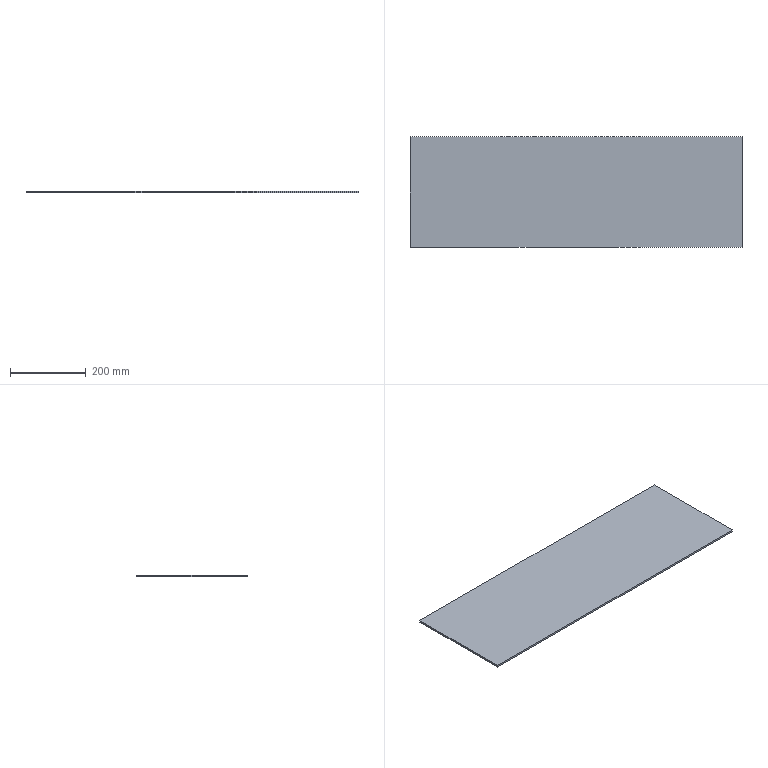Part | SolidWorks | features Extrusion 1, HoleWzd 1 | 1 solid | 6 faces | box 876 x 291 x 5 mm | volume 1274580 mm3 | plane 6
STEP:
#1=CARTESIAN_POINT('',(438.,-145.5,0.));
#2=VERTEX_POINT('',#1);
#3=CARTESIAN_POINT('',(438.,145.5,0.));
#4=VERTEX_POINT('',#3);
#5=CARTESIAN_POINT('',(438.,145.5,0.));
#6=DIRECTION('',(0.,1.,0.));
#7=VECTOR('',#6,1000.);
#8=LINE('',#5,#7);
#9=EDGE_CURVE('',#2,#4,#8,.T.);
#10=ORIENTED_EDGE('',*,*,#9,.T.);
#11=CARTESIAN_POINT('',(438.,145.5,5.));
#12=VERTEX_POINT('',#11);
#13=CARTESIAN_POINT('',(438.,145.5,5.));
#14=DIRECTION('',(0.,0.,-1.));
#15=VECTOR('',#14,1000.);
#16=LINE('',#13,#15);
#17=EDGE_CURVE('',#12,#4,#16,.T.);
#18=ORIENTED_EDGE('',*,*,#17,.F.);
#19=CARTESIAN_POINT('',(438.,-145.5,5.));
#20=VERTEX_POINT('',#19);
#21=CARTESIAN_POINT('',(438.,145.5,5.));
#22=DIRECTION('',(0.,1.,0.));
#23=VECTOR('',#22,1000.);
#24=LINE('',#21,#23);
#25=EDGE_CURVE('',#20,#12,#24,.T.);
#26=ORIENTED_EDGE('',*,*,#25,.F.);
#27=CARTESIAN_POINT('',(438.,-145.5,5.));
#28=DIRECTION('',(0.,0.,-1.));
#29=VECTOR('',#28,1000.);
#30=LINE('',#27,#29);
#31=EDGE_CURVE('',#20,#2,#30,.T.);
#32=ORIENTED_EDGE('',*,*,#31,.T.);
#33=EDGE_LOOP('',(#10,#18,#26,#32));
#34=FACE_OUTER_BOUND('',#33,.T.);
#35=CARTESIAN_POINT('',(438.,145.5,5.));
#36=DIRECTION('',(-1.,0.,0.));
#37=DIRECTION('',(0.,-1.,0.));
#38=AXIS2_PLACEMENT_3D('',#35,#36,#37);
#39=PLANE('',#38);
#40=ADVANCED_FACE('',(#34),#39,.F.);
#41=CARTESIAN_POINT('',(-438.,145.5,0.));
#42=VERTEX_POINT('',#41);
#43=CARTESIAN_POINT('',(-438.,145.5,0.));
#44=DIRECTION('',(-1.,0.,0.));
#45=VECTOR('',#44,1000.);
#46=LINE('',#43,#45);
#47=EDGE_CURVE('',#4,#42,#46,.T.);
#48=ORIENTED_EDGE('',*,*,#47,.T.);
#49=CARTESIAN_POINT('',(-438.,145.5,5.));
#50=VERTEX_POINT('',#49);
#51=CARTESIAN_POINT('',(-438.,145.5,5.));
#52=DIRECTION('',(0.,0.,-1.));
#53=VECTOR('',#52,1000.);
#54=LINE('',#51,#53);
#55=EDGE_CURVE('',#50,#42,#54,.T.);
#56=ORIENTED_EDGE('',*,*,#55,.F.);
#57=CARTESIAN_POINT('',(-438.,145.5,5.));
#58=DIRECTION('',(-1.,0.,0.));
#59=VECTOR('',#58,1000.);
#60=LINE('',#57,#59);
#61=EDGE_CURVE('',#12,#50,#60,.T.);
#62=ORIENTED_EDGE('',*,*,#61,.F.);
#63=ORIENTED_EDGE('',*,*,#17,.T.);
#64=EDGE_LOOP('',(#48,#56,#62,#63));
#65=FACE_OUTER_BOUND('',#64,.T.);
#66=CARTESIAN_POINT('',(-438.,145.5,5.));
#67=DIRECTION('',(0.,-1.,0.));
#68=DIRECTION('',(0.,0.,-1.));
#69=AXIS2_PLACEMENT_3D('',#66,#67,#68);
#70=PLANE('',#69);
#71=ADVANCED_FACE('',(#65),#70,.F.);
#72=CARTESIAN_POINT('',(-438.,-145.5,0.));
#73=VERTEX_POINT('',#72);
#74=CARTESIAN_POINT('',(-438.,145.5,0.));
#75=DIRECTION('',(0.,-1.,0.));
#76=VECTOR('',#75,1000.);
#77=LINE('',#74,#76);
#78=EDGE_CURVE('',#42,#73,#77,.T.);
#79=ORIENTED_EDGE('',*,*,#78,.T.);
#80=CARTESIAN_POINT('',(-438.,-145.5,5.));
#81=VERTEX_POINT('',#80);
#82=CARTESIAN_POINT('',(-438.,-145.5,5.));
#83=DIRECTION('',(0.,0.,-1.));
#84=VECTOR('',#83,1000.);
#85=LINE('',#82,#84);
#86=EDGE_CURVE('',#81,#73,#85,.T.);
#87=ORIENTED_EDGE('',*,*,#86,.F.);
#88=CARTESIAN_POINT('',(-438.,145.5,5.));
#89=DIRECTION('',(0.,-1.,0.));
#90=VECTOR('',#89,1000.);
#91=LINE('',#88,#90);
#92=EDGE_CURVE('',#50,#81,#91,.T.);
#93=ORIENTED_EDGE('',*,*,#92,.F.);
#94=ORIENTED_EDGE('',*,*,#55,.T.);
#95=EDGE_LOOP('',(#79,#87,#93,#94));
#96=FACE_OUTER_BOUND('',#95,.T.);
#97=CARTESIAN_POINT('',(-438.,145.5,5.));
#98=DIRECTION('',(1.,0.,0.));
#99=DIRECTION('',(0.,1.,0.));
#100=AXIS2_PLACEMENT_3D('',#97,#98,#99);
#101=PLANE('',#100);
#102=ADVANCED_FACE('',(#96),#101,.F.);
#103=CARTESIAN_POINT('',(-438.,-145.5,0.));
#104=DIRECTION('',(1.,0.,0.));
#105=VECTOR('',#104,1000.);
#106=LINE('',#103,#105);
#107=EDGE_CURVE('',#73,#2,#106,.T.);
#108=ORIENTED_EDGE('',*,*,#107,.T.);
#109=ORIENTED_EDGE('',*,*,#31,.F.);
#110=CARTESIAN_POINT('',(-438.,-145.5,5.));
#111=DIRECTION('',(1.,0.,0.));
#112=VECTOR('',#111,1000.);
#113=LINE('',#110,#112);
#114=EDGE_CURVE('',#81,#20,#113,.T.);
#115=ORIENTED_EDGE('',*,*,#114,.F.);
#116=ORIENTED_EDGE('',*,*,#86,.T.);
#117=EDGE_LOOP('',(#108,#109,#115,#116));
#118=FACE_OUTER_BOUND('',#117,.T.);
#119=CARTESIAN_POINT('',(-438.,-145.5,5.));
#120=DIRECTION('',(0.,1.,0.));
#121=DIRECTION('',(0.,0.,1.));
#122=AXIS2_PLACEMENT_3D('',#119,#120,#121);
#123=PLANE('',#122);
#124=ADVANCED_FACE('',(#118),#123,.F.);
#125=ORIENTED_EDGE('',*,*,#25,.T.);
#126=ORIENTED_EDGE('',*,*,#61,.T.);
#127=ORIENTED_EDGE('',*,*,#92,.T.);
#128=ORIENTED_EDGE('',*,*,#114,.T.);
#129=EDGE_LOOP('',(#125,#126,#127,#128));
#130=FACE_OUTER_BOUND('',#129,.T.);
#131=CARTESIAN_POINT('',(0.,0.,5.));
#132=DIRECTION('',(0.,0.,1.));
#133=DIRECTION('',(1.,0.,0.));
#134=AXIS2_PLACEMENT_3D('',#131,#132,#133);
#135=PLANE('',#134);
#136=ADVANCED_FACE('',(#130),#135,.T.);
#137=ORIENTED_EDGE('',*,*,#9,.F.);
#138=ORIENTED_EDGE('',*,*,#107,.F.);
#139=ORIENTED_EDGE('',*,*,#78,.F.);
#140=ORIENTED_EDGE('',*,*,#47,.F.);
#141=EDGE_LOOP('',(#137,#138,#139,#140));
#142=FACE_OUTER_BOUND('',#141,.T.);
#143=CARTESIAN_POINT('',(0.,0.,0.));
#144=DIRECTION('',(0.,0.,1.));
#145=DIRECTION('',(1.,0.,0.));
#146=AXIS2_PLACEMENT_3D('',#143,#144,#145);
#147=PLANE('',#146);
#148=ADVANCED_FACE('',(#142),#147,.F.);
#149=CLOSED_SHELL('',(#40,#71,#102,#124,#136,#148));
#150=MANIFOLD_SOLID_BREP('',#149);
#151=CARTESIAN_POINT('',(0.,0.,0.));
#152=DIRECTION('',(0.,0.,1.));
#153=DIRECTION('',(1.,0.,0.));
#154=AXIS2_PLACEMENT_3D('',#151,#152,#153);
#155=(LENGTH_UNIT()NAMED_UNIT(*)SI_UNIT(.MILLI.,.METRE.));
#156=UNCERTAINTY_MEASURE_WITH_UNIT(LENGTH_MEASURE(0.00001),#155,'','');
#157=(NAMED_UNIT(*)PLANE_ANGLE_UNIT()SI_UNIT($,.RADIAN.));
#158=(NAMED_UNIT(*)SI_UNIT($,.STERADIAN.)SOLID_ANGLE_UNIT());
#159=(GEOMETRIC_REPRESENTATION_CONTEXT(3)GLOBAL_UNCERTAINTY_ASSIGNED_CONTEXT((#156))GLOBAL_UNIT_ASSIGNED_CONTEXT((#155,#157,#158))REPRESENTATION_CONTEXT('',''));
#160=ADVANCED_BREP_SHAPE_REPRESENTATION('',(#150,#154),#159);